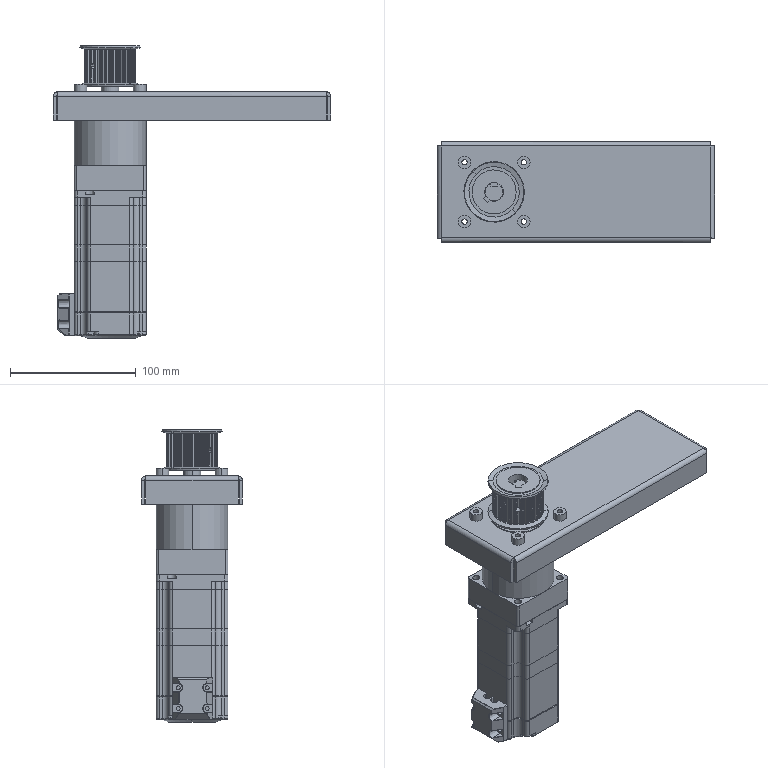Part | SolidWorks | 13 solids | 921 faces | box 220 x 80 x 232.061 mm | volume 626887 mm3 | cylinder 510 | plane 287 | torus 40 | spline 38 | cone 28 | sphere 18 | commonest cylinder face diameters 0.5 x56 6.55 x56 1.1 x52 6 x48 0.4 x42 2 x36